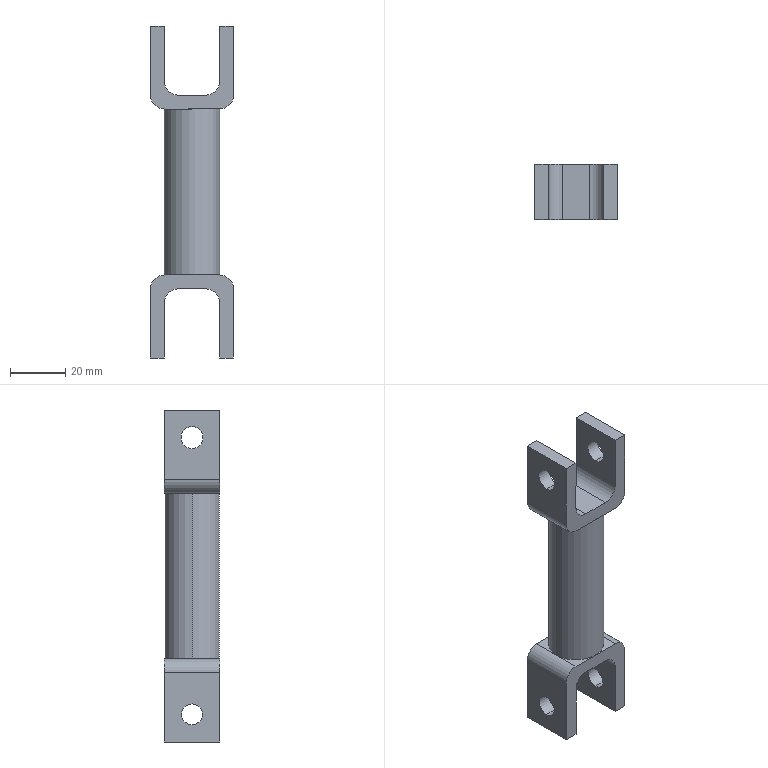Part | SolidWorks | features ICE 2, Extrusion 1 | 3 solids | 40 faces | box 30 x 20 x 120 mm | volume 33900 mm3 | plane 22 | cylinder 18 | commonest cylinder face diameters 10 x8 7.569 x4 7.979 x4 20 x2
STEP:
#1=CARTESIAN_POINT('',(10.,0.,60.));
#2=VERTEX_POINT('',#1);
#3=CARTESIAN_POINT('',(-10.,0.,60.));
#4=VERTEX_POINT('',#3);
#5=CARTESIAN_POINT('',(0.,0.,60.));
#6=DIRECTION('',(0.,0.,1.));
#7=DIRECTION('',(1.,0.,0.));
#8=AXIS2_PLACEMENT_3D('',#5,#6,#7);
#9=CIRCLE('',#8,10.);
#10=EDGE_CURVE('',#2,#4,#9,.T.);
#11=ORIENTED_EDGE('',*,*,#10,.F.);
#12=CARTESIAN_POINT('',(10.,0.,0.));
#13=VERTEX_POINT('',#12);
#14=CARTESIAN_POINT('',(10.,0.,60.));
#15=DIRECTION('',(0.,0.,-1.));
#16=VECTOR('',#15,1000.);
#17=LINE('',#14,#16);
#18=EDGE_CURVE('',#2,#13,#17,.T.);
#19=ORIENTED_EDGE('',*,*,#18,.T.);
#20=CARTESIAN_POINT('',(-10.,0.,0.));
#21=VERTEX_POINT('',#20);
#22=CARTESIAN_POINT('',(0.,0.,0.));
#23=DIRECTION('',(0.,0.,1.));
#24=DIRECTION('',(1.,0.,0.));
#25=AXIS2_PLACEMENT_3D('',#22,#23,#24);
#26=CIRCLE('',#25,10.);
#27=EDGE_CURVE('',#13,#21,#26,.T.);
#28=ORIENTED_EDGE('',*,*,#27,.T.);
#29=CARTESIAN_POINT('',(-10.,0.,60.));
#30=DIRECTION('',(0.,0.,-1.));
#31=VECTOR('',#30,1000.);
#32=LINE('',#29,#31);
#33=EDGE_CURVE('',#4,#21,#32,.T.);
#34=ORIENTED_EDGE('',*,*,#33,.F.);
#35=EDGE_LOOP('',(#11,#19,#28,#34));
#36=FACE_OUTER_BOUND('',#35,.T.);
#37=CARTESIAN_POINT('',(0.,0.,60.));
#38=DIRECTION('',(0.,0.,-1.));
#39=DIRECTION('',(-1.,0.,0.));
#40=AXIS2_PLACEMENT_3D('',#37,#38,#39);
#41=CYLINDRICAL_SURFACE('',#40,10.);
#42=ADVANCED_FACE('',(#36),#41,.T.);
#43=ORIENTED_EDGE('',*,*,#18,.F.);
#44=CARTESIAN_POINT('',(0.,0.,60.));
#45=DIRECTION('',(0.,0.,1.));
#46=DIRECTION('',(1.,0.,0.));
#47=AXIS2_PLACEMENT_3D('',#44,#45,#46);
#48=CIRCLE('',#47,10.);
#49=EDGE_CURVE('',#4,#2,#48,.T.);
#50=ORIENTED_EDGE('',*,*,#49,.F.);
#51=ORIENTED_EDGE('',*,*,#33,.T.);
#52=CARTESIAN_POINT('',(0.,0.,0.));
#53=DIRECTION('',(0.,0.,1.));
#54=DIRECTION('',(1.,0.,0.));
#55=AXIS2_PLACEMENT_3D('',#52,#53,#54);
#56=CIRCLE('',#55,10.);
#57=EDGE_CURVE('',#21,#13,#56,.T.);
#58=ORIENTED_EDGE('',*,*,#57,.T.);
#59=EDGE_LOOP('',(#43,#50,#51,#58));
#60=FACE_OUTER_BOUND('',#59,.T.);
#61=CARTESIAN_POINT('',(0.,0.,60.));
#62=DIRECTION('',(0.,0.,-1.));
#63=DIRECTION('',(-1.,0.,0.));
#64=AXIS2_PLACEMENT_3D('',#61,#62,#63);
#65=CYLINDRICAL_SURFACE('',#64,10.);
#66=ADVANCED_FACE('',(#60),#65,.T.);
#67=ORIENTED_EDGE('',*,*,#49,.T.);
#68=ORIENTED_EDGE('',*,*,#10,.T.);
#69=EDGE_LOOP('',(#67,#68));
#70=FACE_OUTER_BOUND('',#69,.T.);
#71=CARTESIAN_POINT('',(0.,0.,60.));
#72=DIRECTION('',(0.,0.,1.));
#73=DIRECTION('',(1.,0.,0.));
#74=AXIS2_PLACEMENT_3D('',#71,#72,#73);
#75=PLANE('',#74);
#76=ADVANCED_FACE('',(#70),#75,.T.);
#77=ORIENTED_EDGE('',*,*,#57,.F.);
#78=ORIENTED_EDGE('',*,*,#27,.F.);
#79=EDGE_LOOP('',(#77,#78));
#80=FACE_OUTER_BOUND('',#79,.T.);
#81=CARTESIAN_POINT('',(0.,0.,0.));
#82=DIRECTION('',(0.,0.,1.));
#83=DIRECTION('',(1.,0.,0.));
#84=AXIS2_PLACEMENT_3D('',#81,#82,#83);
#85=PLANE('',#84);
#86=ADVANCED_FACE('',(#80),#85,.F.);
#87=CLOSED_SHELL('',(#42,#66,#76,#86));
#88=MANIFOLD_SOLID_BREP('',#87);
#89=CARTESIAN_POINT('',(15.,0.,76.011));
#90=VERTEX_POINT('',#89);
#91=CARTESIAN_POINT('',(15.,0.,83.989));
#92=VERTEX_POINT('',#91);
#93=CARTESIAN_POINT('',(15.,0.,80.));
#94=DIRECTION('',(-1.,0.,0.));
#95=DIRECTION('',(0.,0.,1.));
#96=AXIS2_PLACEMENT_3D('',#93,#94,#95);
#97=CIRCLE('',#96,3.989);
#98=EDGE_CURVE('',#90,#92,#97,.T.);
#99=ORIENTED_EDGE('',*,*,#98,.F.);
#100=CARTESIAN_POINT('',(10.,0.,76.011));
#101=VERTEX_POINT('',#100);
#102=CARTESIAN_POINT('',(15.,0.,76.011));
#103=DIRECTION('',(-1.,0.,0.));
#104=VECTOR('',#103,1000.);
#105=LINE('',#102,#104);
#106=EDGE_CURVE('',#90,#101,#105,.T.);
#107=ORIENTED_EDGE('',*,*,#106,.T.);
#108=CARTESIAN_POINT('',(10.,0.,83.989));
#109=VERTEX_POINT('',#108);
#110=CARTESIAN_POINT('',(10.,0.,80.));
#111=DIRECTION('',(1.,0.,0.));
#112=DIRECTION('',(0.,0.,-1.));
#113=AXIS2_PLACEMENT_3D('',#110,#111,#112);
#114=CIRCLE('',#113,3.989);
#115=EDGE_CURVE('',#109,#101,#114,.T.);
#116=ORIENTED_EDGE('',*,*,#115,.F.);
#117=CARTESIAN_POINT('',(15.,0.,83.989));
#118=DIRECTION('',(-1.,0.,0.));
#119=VECTOR('',#118,1000.);
#120=LINE('',#117,#119);
#121=EDGE_CURVE('',#92,#109,#120,.T.);
#122=ORIENTED_EDGE('',*,*,#121,.F.);
#123=EDGE_LOOP('',(#99,#107,#116,#122));
#124=FACE_OUTER_BOUND('',#123,.T.);
#125=CARTESIAN_POINT('',(15.,0.,80.));
#126=DIRECTION('',(-1.,0.,0.));
#127=DIRECTION('',(0.,0.,1.));
#128=AXIS2_PLACEMENT_3D('',#125,#126,#127);
#129=CYLINDRICAL_SURFACE('',#128,3.989);
#130=ADVANCED_FACE('',(#124),#129,.F.);
#131=CARTESIAN_POINT('',(-10.,0.,76.011));
#132=VERTEX_POINT('',#131);
#133=CARTESIAN_POINT('',(-10.,0.,83.989));
#134=VERTEX_POINT('',#133);
#135=CARTESIAN_POINT('',(-10.,0.,80.));
#136=DIRECTION('',(-1.,0.,0.));
#137=DIRECTION('',(0.,0.,1.));
#138=AXIS2_PLACEMENT_3D('',#135,#136,#137);
#139=CIRCLE('',#138,3.989);
#140=EDGE_CURVE('',#132,#134,#139,.T.);
#141=ORIENTED_EDGE('',*,*,#140,.F.);
#142=CARTESIAN_POINT('',(-15.,0.,76.011));
#143=VERTEX_POINT('',#142);
#144=CARTESIAN_POINT('',(15.,0.,76.011));
#145=DIRECTION('',(-1.,0.,0.));
#146=VECTOR('',#145,1000.);
#147=LINE('',#144,#146);
#148=EDGE_CURVE('',#132,#143,#147,.T.);
#149=ORIENTED_EDGE('',*,*,#148,.T.);
#150=CARTESIAN_POINT('',(-15.,0.,83.989));
#151=VERTEX_POINT('',#150);
#152=CARTESIAN_POINT('',(-15.,0.,80.));
#153=DIRECTION('',(-1.,0.,0.));
#154=DIRECTION('',(0.,0.,1.));
#155=AXIS2_PLACEMENT_3D('',#152,#153,#154);
#156=CIRCLE('',#155,3.989);
#157=EDGE_CURVE('',#143,#151,#156,.T.);
#158=ORIENTED_EDGE('',*,*,#157,.T.);
#159=CARTESIAN_POINT('',(15.,0.,83.989));
#160=DIRECTION('',(-1.,0.,0.));
#161=VECTOR('',#160,1000.);
#162=LINE('',#159,#161);
#163=EDGE_CURVE('',#134,#151,#162,.T.);
#164=ORIENTED_EDGE('',*,*,#163,.F.);
#165=EDGE_LOOP('',(#141,#149,#158,#164));
#166=FACE_OUTER_BOUND('',#165,.T.);
#167=CARTESIAN_POINT('',(15.,0.,80.));
#168=DIRECTION('',(-1.,0.,0.));
#169=DIRECTION('',(0.,0.,1.));
#170=AXIS2_PLACEMENT_3D('',#167,#168,#169);
#171=CYLINDRICAL_SURFACE('',#170,3.989);
#172=ADVANCED_FACE('',(#166),#171,.F.);
#173=CARTESIAN_POINT('',(5.,-10.,65.));
#174=VERTEX_POINT('',#173);
#175=CARTESIAN_POINT('',(10.,-10.,70.));
#176=VERTEX_POINT('',#175);
#177=CARTESIAN_POINT('',(5.,-10.,70.));
#178=DIRECTION('',(0.,-1.,0.));
#179=DIRECTION('',(0.,0.,-1.));
#180=AXIS2_PLACEMENT_3D('',#177,#178,#179);
#181=CIRCLE('',#180,5.);
#182=EDGE_CURVE('',#174,#176,#181,.T.);
#183=ORIENTED_EDGE('',*,*,#182,.T.);
#184=CARTESIAN_POINT('',(10.,10.,70.));
#185=VERTEX_POINT('',#184);
#186=CARTESIAN_POINT('',(10.,10.,70.));
#187=DIRECTION('',(0.,-1.,0.));
#188=VECTOR('',#187,1000.);
#189=LINE('',#186,#188);
#190=EDGE_CURVE('',#185,#176,#189,.T.);
#191=ORIENTED_EDGE('',*,*,#190,.F.);
#192=CARTESIAN_POINT('',(5.,10.,65.));
#193=VERTEX_POINT('',#192);
#194=CARTESIAN_POINT('',(5.,10.,70.));
#195=DIRECTION('',(0.,-1.,0.));
#196=DIRECTION('',(0.,0.,-1.));
#197=AXIS2_PLACEMENT_3D('',#194,#195,#196);
#198=CIRCLE('',#197,5.);
#199=EDGE_CURVE('',#193,#185,#198,.T.);
#200=ORIENTED_EDGE('',*,*,#199,.F.);
#201=CARTESIAN_POINT('',(5.,10.,65.));
#202=DIRECTION('',(0.,-1.,0.));
#203=VECTOR('',#202,1000.);
#204=LINE('',#201,#203);
#205=EDGE_CURVE('',#193,#174,#204,.T.);
#206=ORIENTED_EDGE('',*,*,#205,.T.);
#207=EDGE_LOOP('',(#183,#191,#200,#206));
#208=FACE_OUTER_BOUND('',#207,.T.);
#209=CARTESIAN_POINT('',(5.,10.,70.));
#210=DIRECTION('',(0.,-1.,0.));
#211=DIRECTION('',(0.,0.,-1.));
#212=AXIS2_PLACEMENT_3D('',#209,#210,#211);
#213=CYLINDRICAL_SURFACE('',#212,5.);
#214=ADVANCED_FACE('',(#208),#213,.F.);
#215=ORIENTED_EDGE('',*,*,#115,.T.);
#216=CARTESIAN_POINT('',(10.,0.,80.));
#217=DIRECTION('',(1.,0.,0.));
#218=DIRECTION('',(0.,0.,-1.));
#219=AXIS2_PLACEMENT_3D('',#216,#217,#218);
#220=CIRCLE('',#219,3.989);
#221=EDGE_CURVE('',#101,#109,#220,.T.);
#222=ORIENTED_EDGE('',*,*,#221,.T.);
#223=EDGE_LOOP('',(#215,#222));
#224=FACE_BOUND('',#223,.T.);
#225=CARTESIAN_POINT('',(10.,-10.,90.));
#226=VERTEX_POINT('',#225);
#227=CARTESIAN_POINT('',(10.,-10.,70.));
#228=DIRECTION('',(0.,0.,1.));
#229=VECTOR('',#228,1000.);
#230=LINE('',#227,#229);
#231=EDGE_CURVE('',#176,#226,#230,.T.);
#232=ORIENTED_EDGE('',*,*,#231,.T.);
#233=CARTESIAN_POINT('',(10.,10.,90.));
#234=VERTEX_POINT('',#233);
#235=CARTESIAN_POINT('',(10.,10.,90.));
#236=DIRECTION('',(0.,-1.,0.));
#237=VECTOR('',#236,1000.);
#238=LINE('',#235,#237);
#239=EDGE_CURVE('',#234,#226,#238,.T.);
#240=ORIENTED_EDGE('',*,*,#239,.F.);
#241=CARTESIAN_POINT('',(10.,10.,70.));
#242=DIRECTION('',(0.,0.,1.));
#243=VECTOR('',#242,1000.);
#244=LINE('',#241,#243);
#245=EDGE_CURVE('',#185,#234,#244,.T.);
#246=ORIENTED_EDGE('',*,*,#245,.F.);
#247=ORIENTED_EDGE('',*,*,#190,.T.);
#248=EDGE_LOOP('',(#232,#240,#246,#247));
#249=FACE_OUTER_BOUND('',#248,.T.);
#250=CARTESIAN_POINT('',(10.,10.,70.));
#251=DIRECTION('',(1.,0.,0.));
#252=DIRECTION('',(0.,0.,-1.));
#253=AXIS2_PLACEMENT_3D('',#250,#251,#252);
#254=PLANE('',#253);
#255=ADVANCED_FACE('',(#224,#249),#254,.F.);
#256=CARTESIAN_POINT('',(15.,-10.,90.));
#257=VERTEX_POINT('',#256);
#258=CARTESIAN_POINT('',(10.,-10.,90.));
#259=DIRECTION('',(1.,0.,0.));
#260=VECTOR('',#259,1000.);
#261=LINE('',#258,#260);
#262=EDGE_CURVE('',#226,#257,#261,.T.);
#263=ORIENTED_EDGE('',*,*,#262,.T.);
#264=CARTESIAN_POINT('',(15.,10.,90.));
#265=VERTEX_POINT('',#264);
#266=CARTESIAN_POINT('',(15.,10.,90.));
#267=DIRECTION('',(0.,-1.,0.));
#268=VECTOR('',#267,1000.);
#269=LINE('',#266,#268);
#270=EDGE_CURVE('',#265,#257,#269,.T.);
#271=ORIENTED_EDGE('',*,*,#270,.F.);
#272=CARTESIAN_POINT('',(10.,10.,90.));
#273=DIRECTION('',(1.,0.,0.));
#274=VECTOR('',#273,1000.);
#275=LINE('',#272,#274);
#276=EDGE_CURVE('',#234,#265,#275,.T.);
#277=ORIENTED_EDGE('',*,*,#276,.F.);
#278=ORIENTED_EDGE('',*,*,#239,.T.);
#279=EDGE_LOOP('',(#263,#271,#277,#278));
#280=FACE_OUTER_BOUND('',#279,.T.);
#281=CARTESIAN_POINT('',(10.,10.,90.));
#282=DIRECTION('',(0.,0.,-1.));
#283=DIRECTION('',(-1.,0.,0.));
#284=AXIS2_PLACEMENT_3D('',#281,#282,#283);
#285=PLANE('',#284);
#286=ADVANCED_FACE('',(#280),#285,.F.);
#287=CARTESIAN_POINT('',(15.,0.,80.));
#288=DIRECTION('',(-1.,0.,0.));
#289=DIRECTION('',(0.,0.,1.));
#290=AXIS2_PLACEMENT_3D('',#287,#288,#289);
#291=CIRCLE('',#290,3.989);
#292=EDGE_CURVE('',#92,#90,#291,.T.);
#293=ORIENTED_EDGE('',*,*,#292,.T.);
#294=ORIENTED_EDGE('',*,*,#98,.T.);
#295=EDGE_LOOP('',(#293,#294));
#296=FACE_BOUND('',#295,.T.);
#297=CARTESIAN_POINT('',(15.,-10.,65.));
#298=VERTEX_POINT('',#297);
#299=CARTESIAN_POINT('',(15.,-10.,90.));
#300=DIRECTION('',(0.,0.,-1.));
#301=VECTOR('',#300,1000.);
#302=LINE('',#299,#301);
#303=EDGE_CURVE('',#257,#298,#302,.T.);
#304=ORIENTED_EDGE('',*,*,#303,.T.);
#305=CARTESIAN_POINT('',(15.,10.,65.));
#306=VERTEX_POINT('',#305);
#307=CARTESIAN_POINT('',(15.,10.,65.));
#308=DIRECTION('',(0.,-1.,0.));
#309=VECTOR('',#308,1000.);
#310=LINE('',#307,#309);
#311=EDGE_CURVE('',#306,#298,#310,.T.);
#312=ORIENTED_EDGE('',*,*,#311,.F.);
#313=CARTESIAN_POINT('',(15.,10.,90.));
#314=DIRECTION('',(0.,0.,-1.));
#315=VECTOR('',#314,1000.);
#316=LINE('',#313,#315);
#317=EDGE_CURVE('',#265,#306,#316,.T.);
#318=ORIENTED_EDGE('',*,*,#317,.F.);
#319=ORIENTED_EDGE('',*,*,#270,.T.);
#320=EDGE_LOOP('',(#304,#312,#318,#319));
#321=FACE_OUTER_BOUND('',#320,.T.);
#322=CARTESIAN_POINT('',(15.,10.,90.));
#323=DIRECTION('',(-1.,0.,0.));
#324=DIRECTION('',(0.,0.,1.));
#325=AXIS2_PLACEMENT_3D('',#322,#323,#324);
#326=PLANE('',#325);
#327=ADVANCED_FACE('',(#296,#321),#326,.F.);
#328=CARTESIAN_POINT('',(10.,-10.,60.));
#329=VERTEX_POINT('',#328);
#330=CARTESIAN_POINT('',(10.,-10.,65.));
#331=DIRECTION('',(0.,1.,0.));
#332=DIRECTION('',(0.,0.,-1.));
#333=AXIS2_PLACEMENT_3D('',#330,#331,#332);
#334=CIRCLE('',#333,5.);
#335=EDGE_CURVE('',#298,#329,#334,.T.);
#336=ORIENTED_EDGE('',*,*,#335,.T.);
#337=CARTESIAN_POINT('',(10.,10.,60.));
#338=VERTEX_POINT('',#337);
#339=CARTESIAN_POINT('',(10.,10.,60.));
#340=DIRECTION('',(0.,-1.,0.));
#341=VECTOR('',#340,1000.);
#342=LINE('',#339,#341);
#343=EDGE_CURVE('',#338,#329,#342,.T.);
#344=ORIENTED_EDGE('',*,*,#343,.F.);
#345=CARTESIAN_POINT('',(10.,10.,65.));
#346=DIRECTION('',(0.,1.,0.));
#347=DIRECTION('',(0.,0.,-1.));
#348=AXIS2_PLACEMENT_3D('',#345,#346,#347);
#349=CIRCLE('',#348,5.);
#350=EDGE_CURVE('',#306,#338,#349,.T.);
#351=ORIENTED_EDGE('',*,*,#350,.F.);
#352=ORIENTED_EDGE('',*,*,#311,.T.);
#353=EDGE_LOOP('',(#336,#344,#351,#352));
#354=FACE_OUTER_BOUND('',#353,.T.);
#355=CARTESIAN_POINT('',(10.,10.,65.));
#356=DIRECTION('',(0.,-1.,0.));
#357=DIRECTION('',(0.,0.,-1.));
#358=AXIS2_PLACEMENT_3D('',#355,#356,#357);
#359=CYLINDRICAL_SURFACE('',#358,5.);
#360=ADVANCED_FACE('',(#354),#359,.T.);
#361=CARTESIAN_POINT('',(-10.,-10.,60.));
#362=VERTEX_POINT('',#361);
#363=CARTESIAN_POINT('',(-10.,-10.,60.));
#364=DIRECTION('',(-1.,0.,0.));
#365=VECTOR('',#364,1000.);
#366=LINE('',#363,#365);
#367=EDGE_CURVE('',#329,#362,#366,.T.);
#368=ORIENTED_EDGE('',*,*,#367,.T.);
#369=CARTESIAN_POINT('',(-10.,10.,60.));
#370=VERTEX_POINT('',#369);
#371=CARTESIAN_POINT('',(-10.,10.,60.));
#372=DIRECTION('',(0.,-1.,0.));
#373=VECTOR('',#372,1000.);
#374=LINE('',#371,#373);
#375=EDGE_CURVE('',#370,#362,#374,.T.);
#376=ORIENTED_EDGE('',*,*,#375,.F.);
#377=CARTESIAN_POINT('',(-10.,10.,60.));
#378=DIRECTION('',(-1.,0.,0.));
#379=VECTOR('',#378,1000.);
#380=LINE('',#377,#379);
#381=EDGE_CURVE('',#338,#370,#380,.T.);
#382=ORIENTED_EDGE('',*,*,#381,.F.);
#383=ORIENTED_EDGE('',*,*,#343,.T.);
#384=EDGE_LOOP('',(#368,#376,#382,#383));
#385=FACE_OUTER_BOUND('',#384,.T.);
#386=CARTESIAN_POINT('',(-10.,10.,60.));
#387=DIRECTION('',(0.,0.,1.));
#388=DIRECTION('',(1.,0.,0.));
#389=AXIS2_PLACEMENT_3D('',#386,#387,#388);
#390=PLANE('',#389);
#391=ADVANCED_FACE('',(#385),#390,.F.);
#392=CARTESIAN_POINT('',(-15.,-10.,65.));
#393=VERTEX_POINT('',#392);
#394=CARTESIAN_POINT('',(-10.,-10.,65.));
#395=DIRECTION('',(0.,1.,0.));
#396=DIRECTION('',(0.,0.,-1.));
#397=AXIS2_PLACEMENT_3D('',#394,#395,#396);
#398=CIRCLE('',#397,5.);
#399=EDGE_CURVE('',#362,#393,#398,.T.);
#400=ORIENTED_EDGE('',*,*,#399,.T.);
#401=CARTESIAN_POINT('',(-15.,10.,65.));
#402=VERTEX_POINT('',#401);
#403=CARTESIAN_POINT('',(-15.,10.,65.));
#404=DIRECTION('',(0.,-1.,0.));
#405=VECTOR('',#404,1000.);
#406=LINE('',#403,#405);
#407=EDGE_CURVE('',#402,#393,#406,.T.);
#408=ORIENTED_EDGE('',*,*,#407,.F.);
#409=CARTESIAN_POINT('',(-10.,10.,65.));
#410=DIRECTION('',(0.,1.,0.));
#411=DIRECTION('',(0.,0.,-1.));
#412=AXIS2_PLACEMENT_3D('',#409,#410,#411);
#413=CIRCLE('',#412,5.);
#414=EDGE_CURVE('',#370,#402,#413,.T.);
#415=ORIENTED_EDGE('',*,*,#414,.F.);
#416=ORIENTED_EDGE('',*,*,#375,.T.);
#417=EDGE_LOOP('',(#400,#408,#415,#416));
#418=FACE_OUTER_BOUND('',#417,.T.);
#419=CARTESIAN_POINT('',(-10.,10.,65.));
#420=DIRECTION('',(0.,-1.,0.));
#421=DIRECTION('',(0.,0.,-1.));
#422=AXIS2_PLACEMENT_3D('',#419,#420,#421);
#423=CYLINDRICAL_SURFACE('',#422,5.);
#424=ADVANCED_FACE('',(#418),#423,.T.);
#425=CARTESIAN_POINT('',(-15.,0.,80.));
#426=DIRECTION('',(-1.,0.,0.));
#427=DIRECTION('',(0.,0.,1.));
#428=AXIS2_PLACEMENT_3D('',#425,#426,#427);
#429=CIRCLE('',#428,3.989);
#430=EDGE_CURVE('',#151,#143,#429,.T.);
#431=ORIENTED_EDGE('',*,*,#430,.F.);
#432=ORIENTED_EDGE('',*,*,#157,.F.);
#433=EDGE_LOOP('',(#431,#432));
#434=FACE_BOUND('',#433,.T.);
#435=CARTESIAN_POINT('',(-15.,-10.,90.));
#436=VERTEX_POINT('',#435);
#437=CARTESIAN_POINT('',(-15.,-10.,90.));
#438=DIRECTION('',(0.,0.,1.));
#439=VECTOR('',#438,1000.);
#440=LINE('',#437,#439);
#441=EDGE_CURVE('',#393,#436,#440,.T.);
#442=ORIENTED_EDGE('',*,*,#441,.T.);
#443=CARTESIAN_POINT('',(-15.,10.,90.));
#444=VERTEX_POINT('',#443);
#445=CARTESIAN_POINT('',(-15.,10.,90.));
#446=DIRECTION('',(0.,-1.,0.));
#447=VECTOR('',#446,1000.);
#448=LINE('',#445,#447);
#449=EDGE_CURVE('',#444,#436,#448,.T.);
#450=ORIENTED_EDGE('',*,*,#449,.F.);
#451=CARTESIAN_POINT('',(-15.,10.,90.));
#452=DIRECTION('',(0.,0.,1.));
#453=VECTOR('',#452,1000.);
#454=LINE('',#451,#453);
#455=EDGE_CURVE('',#402,#444,#454,.T.);
#456=ORIENTED_EDGE('',*,*,#455,.F.);
#457=ORIENTED_EDGE('',*,*,#407,.T.);
#458=EDGE_LOOP('',(#442,#450,#456,#457));
#459=FACE_OUTER_BOUND('',#458,.T.);
#460=CARTESIAN_POINT('',(-15.,10.,90.));
#461=DIRECTION('',(1.,0.,0.));
#462=DIRECTION('',(0.,0.,-1.));
#463=AXIS2_PLACEMENT_3D('',#460,#461,#462);
#464=PLANE('',#463);
#465=ADVANCED_FACE('',(#434,#459),#464,.F.);
#466=CARTESIAN_POINT('',(-10.,-10.,90.));
#467=VERTEX_POINT('',#466);
#468=CARTESIAN_POINT('',(-15.,-10.,90.));
#469=DIRECTION('',(1.,0.,0.));
#470=VECTOR('',#469,1000.);
#471=LINE('',#468,#470);
#472=EDGE_CURVE('',#436,#467,#471,.T.);
#473=ORIENTED_EDGE('',*,*,#472,.T.);
#474=CARTESIAN_POINT('',(-10.,10.,90.));
#475=VERTEX_POINT('',#474);
#476=CARTESIAN_POINT('',(-10.,10.,90.));
#477=DIRECTION('',(0.,-1.,0.));
#478=VECTOR('',#477,1000.);
#479=LINE('',#476,#478);
#480=EDGE_CURVE('',#475,#467,#479,.T.);
#481=ORIENTED_EDGE('',*,*,#480,.F.);
#482=CARTESIAN_POINT('',(-15.,10.,90.));
#483=DIRECTION('',(1.,0.,0.));
#484=VECTOR('',#483,1000.);
#485=LINE('',#482,#484);
#486=EDGE_CURVE('',#444,#475,#485,.T.);
#487=ORIENTED_EDGE('',*,*,#486,.F.);
#488=ORIENTED_EDGE('',*,*,#449,.T.);
#489=EDGE_LOOP('',(#473,#481,#487,#488));
#490=FACE_OUTER_BOUND('',#489,.T.);
#491=CARTESIAN_POINT('',(-15.,10.,90.));
#492=DIRECTION('',(0.,0.,-1.));
#493=DIRECTION('',(-1.,0.,0.));
#494=AXIS2_PLACEMENT_3D('',#491,#492,#493);
#495=PLANE('',#494);
#496=ADVANCED_FACE('',(#490),#495,.F.);
#497=CARTESIAN_POINT('',(-10.,0.,80.));
#498=DIRECTION('',(-1.,0.,0.));
#499=DIRECTION('',(0.,0.,1.));
#500=AXIS2_PLACEMENT_3D('',#497,#498,#499);
#501=CIRCLE('',#500,3.989);
#502=EDGE_CURVE('',#134,#132,#501,.T.);
#503=ORIENTED_EDGE('',*,*,#502,.T.);
#504=ORIENTED_EDGE('',*,*,#140,.T.);
#505=EDGE_LOOP('',(#503,#504));
#506=FACE_BOUND('',#505,.T.);
#507=CARTESIAN_POINT('',(-10.,-10.,70.));
#508=VERTEX_POINT('',#507);
#509=CARTESIAN_POINT('',(-10.,-10.,90.));
#510=DIRECTION('',(0.,0.,-1.));
#511=VECTOR('',#510,1000.);
#512=LINE('',#509,#511);
#513=EDGE_CURVE('',#467,#508,#512,.T.);
#514=ORIENTED_EDGE('',*,*,#513,.T.);
#515=CARTESIAN_POINT('',(-10.,10.,70.));
#516=VERTEX_POINT('',#515);
#517=CARTESIAN_POINT('',(-10.,10.,70.));
#518=DIRECTION('',(0.,-1.,0.));
#519=VECTOR('',#518,1000.);
#520=LINE('',#517,#519);
#521=EDGE_CURVE('',#516,#508,#520,.T.);
#522=ORIENTED_EDGE('',*,*,#521,.F.);
#523=CARTESIAN_POINT('',(-10.,10.,90.));
#524=DIRECTION('',(0.,0.,-1.));
#525=VECTOR('',#524,1000.);
#526=LINE('',#523,#525);
#527=EDGE_CURVE('',#475,#516,#526,.T.);
#528=ORIENTED_EDGE('',*,*,#527,.F.);
#529=ORIENTED_EDGE('',*,*,#480,.T.);
#530=EDGE_LOOP('',(#514,#522,#528,#529));
#531=FACE_OUTER_BOUND('',#530,.T.);
#532=CARTESIAN_POINT('',(-10.,10.,90.));
#533=DIRECTION('',(-1.,0.,0.));
#534=DIRECTION('',(0.,0.,1.));
#535=AXIS2_PLACEMENT_3D('',#532,#533,#534);
#536=PLANE('',#535);
#537=ADVANCED_FACE('',(#506,#531),#536,.F.);
#538=CARTESIAN_POINT('',(-5.,-10.,65.));
#539=VERTEX_POINT('',#538);
#540=CARTESIAN_POINT('',(-5.,-10.,70.));
#541=DIRECTION('',(0.,-1.,0.));
#542=DIRECTION('',(0.,0.,-1.));
#543=AXIS2_PLACEMENT_3D('',#540,#541,#542);
#544=CIRCLE('',#543,5.);
#545=EDGE_CURVE('',#508,#539,#544,.T.);
#546=ORIENTED_EDGE('',*,*,#545,.T.);
#547=CARTESIAN_POINT('',(-5.,10.,65.));
#548=VERTEX_POINT('',#547);
#549=CARTESIAN_POINT('',(-5.,10.,65.));
#550=DIRECTION('',(0.,-1.,0.));
#551=VECTOR('',#550,1000.);
#552=LINE('',#549,#551);
#553=EDGE_CURVE('',#548,#539,#552,.T.);
#554=ORIENTED_EDGE('',*,*,#553,.F.);
#555=CARTESIAN_POINT('',(-5.,10.,70.));
#556=DIRECTION('',(0.,-1.,0.));
#557=DIRECTION('',(0.,0.,-1.));
#558=AXIS2_PLACEMENT_3D('',#555,#556,#557);
#559=CIRCLE('',#558,5.);
#560=EDGE_CURVE('',#516,#548,#559,.T.);
#561=ORIENTED_EDGE('',*,*,#560,.F.);
#562=ORIENTED_EDGE('',*,*,#521,.T.);
#563=EDGE_LOOP('',(#546,#554,#561,#562));
#564=FACE_OUTER_BOUND('',#563,.T.);
#565=CARTESIAN_POINT('',(-5.,10.,70.));
#566=DIRECTION('',(0.,-1.,0.));
#567=DIRECTION('',(0.,0.,-1.));
#568=AXIS2_PLACEMENT_3D('',#565,#566,#567);
#569=CYLINDRICAL_SURFACE('',#568,5.);
#570=ADVANCED_FACE('',(#564),#569,.F.);
#571=CARTESIAN_POINT('',(-5.,-10.,65.));
#572=DIRECTION('',(1.,0.,0.));
#573=VECTOR('',#572,1000.);
#574=LINE('',#571,#573);
#575=EDGE_CURVE('',#539,#174,#574,.T.);
#576=ORIENTED_EDGE('',*,*,#575,.T.);
#577=ORIENTED_EDGE('',*,*,#205,.F.);
#578=CARTESIAN_POINT('',(-5.,10.,65.));
#579=DIRECTION('',(1.,0.,0.));
#580=VECTOR('',#579,1000.);
#581=LINE('',#578,#580);
#582=EDGE_CURVE('',#548,#193,#581,.T.);
#583=ORIENTED_EDGE('',*,*,#582,.F.);
#584=ORIENTED_EDGE('',*,*,#553,.T.);
#585=EDGE_LOOP('',(#576,#577,#583,#584));
#586=FACE_OUTER_BOUND('',#585,.T.);
#587=CARTESIAN_POINT('',(-5.,10.,65.));
#588=DIRECTION('',(0.,0.,-1.));
#589=DIRECTION('',(-1.,0.,0.));
#590=AXIS2_PLACEMENT_3D('',#587,#588,#589);
#591=PLANE('',#590);
#592=ADVANCED_FACE('',(#586),#591,.F.);
#593=ORIENTED_EDGE('',*,*,#199,.T.);
#594=ORIENTED_EDGE('',*,*,#245,.T.);
#595=ORIENTED_EDGE('',*,*,#276,.T.);
#596=ORIENTED_EDGE('',*,*,#317,.T.);
#597=ORIENTED_EDGE('',*,*,#350,.T.);
#598=ORIENTED_EDGE('',*,*,#381,.T.);
#599=ORIENTED_EDGE('',*,*,#414,.T.);
#600=ORIENTED_EDGE('',*,*,#455,.T.);
#601=ORIENTED_EDGE('',*,*,#486,.T.);
#602=ORIENTED_EDGE('',*,*,#527,.T.);
#603=ORIENTED_EDGE('',*,*,#560,.T.);
#604=ORIENTED_EDGE('',*,*,#582,.T.);
#605=EDGE_LOOP('',(#593,#594,#595,#596,#597,#598,#599,#600,#601,#602,#603,#604));
#606=FACE_OUTER_BOUND('',#605,.T.);
#607=CARTESIAN_POINT('',(5.,10.,70.));
#608=DIRECTION('',(0.,-1.,0.));
#609=DIRECTION('',(0.,0.,-1.));
#610=AXIS2_PLACEMENT_3D('',#607,#608,#609);
#611=PLANE('',#610);
#612=ADVANCED_FACE('',(#606),#611,.F.);
#613=ORIENTED_EDGE('',*,*,#182,.F.);
#614=ORIENTED_EDGE('',*,*,#575,.F.);
#615=ORIENTED_EDGE('',*,*,#545,.F.);
#616=ORIENTED_EDGE('',*,*,#513,.F.);
#617=ORIENTED_EDGE('',*,*,#472,.F.);
#618=ORIENTED_EDGE('',*,*,#441,.F.);
#619=ORIENTED_EDGE('',*,*,#399,.F.);
#620=ORIENTED_EDGE('',*,*,#367,.F.);
#621=ORIENTED_EDGE('',*,*,#335,.F.);
#622=ORIENTED_EDGE('',*,*,#303,.F.);
#623=ORIENTED_EDGE('',*,*,#262,.F.);
#624=ORIENTED_EDGE('',*,*,#231,.F.);
#625=EDGE_LOOP('',(#613,#614,#615,#616,#617,#618,#619,#620,#621,#622,#623,#624));
#626=FACE_OUTER_BOUND('',#625,.T.);
#627=CARTESIAN_POINT('',(5.,-10.,70.));
#628=DIRECTION('',(0.,-1.,0.));
#629=DIRECTION('',(0.,0.,-1.));
#630=AXIS2_PLACEMENT_3D('',#627,#628,#629);
#631=PLANE('',#630);
#632=ADVANCED_FACE('',(#626),#631,.T.);
#633=ORIENTED_EDGE('',*,*,#148,.F.);
#634=ORIENTED_EDGE('',*,*,#502,.F.);
#635=ORIENTED_EDGE('',*,*,#163,.T.);
#636=ORIENTED_EDGE('',*,*,#430,.T.);
#637=EDGE_LOOP('',(#633,#634,#635,#636));
#638=FACE_OUTER_BOUND('',#637,.T.);
#639=CARTESIAN_POINT('',(15.,0.,80.));
#640=DIRECTION('',(-1.,0.,0.));
#641=DIRECTION('',(0.,0.,1.));
#642=AXIS2_PLACEMENT_3D('',#639,#640,#641);
#643=CYLINDRICAL_SURFACE('',#642,3.989);
#644=ADVANCED_FACE('',(#638),#643,.F.);
#645=ORIENTED_EDGE('',*,*,#106,.F.);
#646=ORIENTED_EDGE('',*,*,#292,.F.);
#647=ORIENTED_EDGE('',*,*,#121,.T.);
#648=ORIENTED_EDGE('',*,*,#221,.F.);
#649=EDGE_LOOP('',(#645,#646,#647,#648));
#650=FACE_OUTER_BOUND('',#649,.T.);
#651=CARTESIAN_POINT('',(15.,0.,80.));
#652=DIRECTION('',(-1.,0.,0.));
#653=DIRECTION('',(0.,0.,1.));
#654=AXIS2_PLACEMENT_3D('',#651,#652,#653);
#655=CYLINDRICAL_SURFACE('',#654,3.989);
#656=ADVANCED_FACE('',(#650),#655,.F.);
#657=CLOSED_SHELL('',(#130,#172,#214,#255,#286,#327,#360,#391,#424,#465,#496,#537,#570,#592,#612,#632,#644,#656));
#658=MANIFOLD_SOLID_BREP('',#657);
#659=CARTESIAN_POINT('',(15.,0.,-23.784));
#660=VERTEX_POINT('',#659);
#661=CARTESIAN_POINT('',(15.,0.,-16.216));
#662=VERTEX_POINT('',#661);
#663=CARTESIAN_POINT('',(15.,0.,-20.));
#664=DIRECTION('',(-1.,0.,0.));
#665=DIRECTION('',(0.,0.,1.));
#666=AXIS2_PLACEMENT_3D('',#663,#664,#665);
#667=CIRCLE('',#666,3.784);
#668=EDGE_CURVE('',#660,#662,#667,.T.);
#669=ORIENTED_EDGE('',*,*,#668,.F.);
#670=CARTESIAN_POINT('',(10.,0.,-23.784));
#671=VERTEX_POINT('',#670);
#672=CARTESIAN_POINT('',(15.,0.,-23.784));
#673=DIRECTION('',(-1.,0.,0.));
#674=VECTOR('',#673,1000.);
#675=LINE('',#672,#674);
#676=EDGE_CURVE('',#660,#671,#675,.T.);
#677=ORIENTED_EDGE('',*,*,#676,.T.);
#678=CARTESIAN_POINT('',(10.,0.,-16.216));
#679=VERTEX_POINT('',#678);
#680=CARTESIAN_POINT('',(10.,0.,-20.));
#681=DIRECTION('',(1.,0.,0.));
#682=DIRECTION('',(0.,0.,-1.));
#683=AXIS2_PLACEMENT_3D('',#680,#681,#682);
#684=CIRCLE('',#683,3.784);
#685=EDGE_CURVE('',#679,#671,#684,.T.);
#686=ORIENTED_EDGE('',*,*,#685,.F.);
#687=CARTESIAN_POINT('',(15.,0.,-16.216));
#688=DIRECTION('',(-1.,0.,0.));
#689=VECTOR('',#688,1000.);
#690=LINE('',#687,#689);
#691=EDGE_CURVE('',#662,#679,#690,.T.);
#692=ORIENTED_EDGE('',*,*,#691,.F.);
#693=EDGE_LOOP('',(#669,#677,#686,#692));
#694=FACE_OUTER_BOUND('',#693,.T.);
#695=CARTESIAN_POINT('',(15.,0.,-20.));
#696=DIRECTION('',(-1.,0.,0.));
#697=DIRECTION('',(0.,0.,1.));
#698=AXIS2_PLACEMENT_3D('',#695,#696,#697);
#699=CYLINDRICAL_SURFACE('',#698,3.784);
#700=ADVANCED_FACE('',(#694),#699,.F.);
#701=CARTESIAN_POINT('',(-10.,0.,-23.784));
#702=VERTEX_POINT('',#701);
#703=CARTESIAN_POINT('',(-10.,0.,-16.216));
#704=VERTEX_POINT('',#703);
#705=CARTESIAN_POINT('',(-10.,0.,-20.));
#706=DIRECTION('',(-1.,0.,0.));
#707=DIRECTION('',(0.,0.,1.));
#708=AXIS2_PLACEMENT_3D('',#705,#706,#707);
#709=CIRCLE('',#708,3.784);
#710=EDGE_CURVE('',#702,#704,#709,.T.);
#711=ORIENTED_EDGE('',*,*,#710,.F.);
#712=CARTESIAN_POINT('',(-15.,0.,-23.784));
#713=VERTEX_POINT('',#712);
#714=CARTESIAN_POINT('',(15.,0.,-23.784));
#715=DIRECTION('',(-1.,0.,0.));
#716=VECTOR('',#715,1000.);
#717=LINE('',#714,#716);
#718=EDGE_CURVE('',#702,#713,#717,.T.);
#719=ORIENTED_EDGE('',*,*,#718,.T.);
#720=CARTESIAN_POINT('',(-15.,0.,-16.216));
#721=VERTEX_POINT('',#720);
#722=CARTESIAN_POINT('',(-15.,0.,-20.));
#723=DIRECTION('',(-1.,0.,0.));
#724=DIRECTION('',(0.,0.,1.));
#725=AXIS2_PLACEMENT_3D('',#722,#723,#724);
#726=CIRCLE('',#725,3.784);
#727=EDGE_CURVE('',#713,#721,#726,.T.);
#728=ORIENTED_EDGE('',*,*,#727,.T.);
#729=CARTESIAN_POINT('',(15.,0.,-16.216));
#730=DIRECTION('',(-1.,0.,0.));
#731=VECTOR('',#730,1000.);
#732=LINE('',#729,#731);
#733=EDGE_CURVE('',#704,#721,#732,.T.);
#734=ORIENTED_EDGE('',*,*,#733,.F.);
#735=EDGE_LOOP('',(#711,#719,#728,#734));
#736=FACE_OUTER_BOUND('',#735,.T.);
#737=CARTESIAN_POINT('',(15.,0.,-20.));
#738=DIRECTION('',(-1.,0.,0.));
#739=DIRECTION('',(0.,0.,1.));
#740=AXIS2_PLACEMENT_3D('',#737,#738,#739);
#741=CYLINDRICAL_SURFACE('',#740,3.784);
#742=ADVANCED_FACE('',(#736),#741,.F.);
#743=CARTESIAN_POINT('',(-15.,0.,-20.));
#744=DIRECTION('',(-1.,0.,0.));
#745=DIRECTION('',(0.,0.,1.));
#746=AXIS2_PLACEMENT_3D('',#743,#744,#745);
#747=CIRCLE('',#746,3.784);
#748=EDGE_CURVE('',#721,#713,#747,.T.);
#749=ORIENTED_EDGE('',*,*,#748,.F.);
#750=ORIENTED_EDGE('',*,*,#727,.F.);
#751=EDGE_LOOP('',(#749,#750));
#752=FACE_BOUND('',#751,.T.);
#753=CARTESIAN_POINT('',(-15.,-10.,-30.));
#754=VERTEX_POINT('',#753);
#755=CARTESIAN_POINT('',(-15.,-10.,-5.));
#756=VERTEX_POINT('',#755);
#757=CARTESIAN_POINT('',(-15.,-10.,-30.));
#758=DIRECTION('',(0.,0.,1.));
#759=VECTOR('',#758,1000.);
#760=LINE('',#757,#759);
#761=EDGE_CURVE('',#754,#756,#760,.T.);
#762=ORIENTED_EDGE('',*,*,#761,.T.);
#763=CARTESIAN_POINT('',(-15.,10.,-5.));
#764=VERTEX_POINT('',#763);
#765=CARTESIAN_POINT('',(-15.,10.,-5.));
#766=DIRECTION('',(0.,-1.,0.));
#767=VECTOR('',#766,1000.);
#768=LINE('',#765,#767);
#769=EDGE_CURVE('',#764,#756,#768,.T.);
#770=ORIENTED_EDGE('',*,*,#769,.F.);
#771=CARTESIAN_POINT('',(-15.,10.,-30.));
#772=VERTEX_POINT('',#771);
#773=CARTESIAN_POINT('',(-15.,10.,-30.));
#774=DIRECTION('',(0.,0.,1.));
#775=VECTOR('',#774,1000.);
#776=LINE('',#773,#775);
#777=EDGE_CURVE('',#772,#764,#776,.T.);
#778=ORIENTED_EDGE('',*,*,#777,.F.);
#779=CARTESIAN_POINT('',(-15.,10.,-30.));
#780=DIRECTION('',(0.,-1.,0.));
#781=VECTOR('',#780,1000.);
#782=LINE('',#779,#781);
#783=EDGE_CURVE('',#772,#754,#782,.T.);
#784=ORIENTED_EDGE('',*,*,#783,.T.);
#785=EDGE_LOOP('',(#762,#770,#778,#784));
#786=FACE_OUTER_BOUND('',#785,.T.);
#787=CARTESIAN_POINT('',(-15.,10.,-30.));
#788=DIRECTION('',(1.,0.,0.));
#789=DIRECTION('',(0.,0.,-1.));
#790=AXIS2_PLACEMENT_3D('',#787,#788,#789);
#791=PLANE('',#790);
#792=ADVANCED_FACE('',(#752,#786),#791,.F.);
#793=CARTESIAN_POINT('',(-10.,-10.,0.));
#794=VERTEX_POINT('',#793);
#795=CARTESIAN_POINT('',(-10.,-10.,-5.));
#796=DIRECTION('',(0.,1.,0.));
#797=DIRECTION('',(0.,0.,1.));
#798=AXIS2_PLACEMENT_3D('',#795,#796,#797);
#799=CIRCLE('',#798,5.);
#800=EDGE_CURVE('',#756,#794,#799,.T.);
#801=ORIENTED_EDGE('',*,*,#800,.T.);
#802=CARTESIAN_POINT('',(-10.,10.,0.));
#803=VERTEX_POINT('',#802);
#804=CARTESIAN_POINT('',(-10.,10.,0.));
#805=DIRECTION('',(0.,-1.,0.));
#806=VECTOR('',#805,1000.);
#807=LINE('',#804,#806);
#808=EDGE_CURVE('',#803,#794,#807,.T.);
#809=ORIENTED_EDGE('',*,*,#808,.F.);
#810=CARTESIAN_POINT('',(-10.,10.,-5.));
#811=DIRECTION('',(0.,1.,0.));
#812=DIRECTION('',(0.,0.,1.));
#813=AXIS2_PLACEMENT_3D('',#810,#811,#812);
#814=CIRCLE('',#813,5.);
#815=EDGE_CURVE('',#764,#803,#814,.T.);
#816=ORIENTED_EDGE('',*,*,#815,.F.);
#817=ORIENTED_EDGE('',*,*,#769,.T.);
#818=EDGE_LOOP('',(#801,#809,#816,#817));
#819=FACE_OUTER_BOUND('',#818,.T.);
#820=CARTESIAN_POINT('',(-10.,10.,-5.));
#821=DIRECTION('',(0.,-1.,0.));
#822=DIRECTION('',(0.,0.,-1.));
#823=AXIS2_PLACEMENT_3D('',#820,#821,#822);
#824=CYLINDRICAL_SURFACE('',#823,5.);
#825=ADVANCED_FACE('',(#819),#824,.T.);
#826=CARTESIAN_POINT('',(10.,-10.,0.));
#827=VERTEX_POINT('',#826);
#828=CARTESIAN_POINT('',(-10.,-10.,0.));
#829=DIRECTION('',(1.,0.,0.));
#830=VECTOR('',#829,1000.);
#831=LINE('',#828,#830);
#832=EDGE_CURVE('',#794,#827,#831,.T.);
#833=ORIENTED_EDGE('',*,*,#832,.T.);
#834=CARTESIAN_POINT('',(10.,10.,0.));
#835=VERTEX_POINT('',#834);
#836=CARTESIAN_POINT('',(10.,10.,0.));
#837=DIRECTION('',(0.,-1.,0.));
#838=VECTOR('',#837,1000.);
#839=LINE('',#836,#838);
#840=EDGE_CURVE('',#835,#827,#839,.T.);
#841=ORIENTED_EDGE('',*,*,#840,.F.);
#842=CARTESIAN_POINT('',(-10.,10.,0.));
#843=DIRECTION('',(1.,0.,0.));
#844=VECTOR('',#843,1000.);
#845=LINE('',#842,#844);
#846=EDGE_CURVE('',#803,#835,#845,.T.);
#847=ORIENTED_EDGE('',*,*,#846,.F.);
#848=ORIENTED_EDGE('',*,*,#808,.T.);
#849=EDGE_LOOP('',(#833,#841,#847,#848));
#850=FACE_OUTER_BOUND('',#849,.T.);
#851=CARTESIAN_POINT('',(-10.,10.,0.));
#852=DIRECTION('',(0.,0.,-1.));
#853=DIRECTION('',(-1.,0.,0.));
#854=AXIS2_PLACEMENT_3D('',#851,#852,#853);
#855=PLANE('',#854);
#856=ADVANCED_FACE('',(#850),#855,.F.);
#857=CARTESIAN_POINT('',(15.,-10.,-5.));
#858=VERTEX_POINT('',#857);
#859=CARTESIAN_POINT('',(10.,-10.,-5.));
#860=DIRECTION('',(0.,1.,0.));
#861=DIRECTION('',(0.,0.,1.));
#862=AXIS2_PLACEMENT_3D('',#859,#860,#861);
#863=CIRCLE('',#862,5.);
#864=EDGE_CURVE('',#827,#858,#863,.T.);
#865=ORIENTED_EDGE('',*,*,#864,.T.);
#866=CARTESIAN_POINT('',(15.,10.,-5.));
#867=VERTEX_POINT('',#866);
#868=CARTESIAN_POINT('',(15.,10.,-5.));
#869=DIRECTION('',(0.,-1.,0.));
#870=VECTOR('',#869,1000.);
#871=LINE('',#868,#870);
#872=EDGE_CURVE('',#867,#858,#871,.T.);
#873=ORIENTED_EDGE('',*,*,#872,.F.);
#874=CARTESIAN_POINT('',(10.,10.,-5.));
#875=DIRECTION('',(0.,1.,0.));
#876=DIRECTION('',(0.,0.,1.));
#877=AXIS2_PLACEMENT_3D('',#874,#875,#876);
#878=CIRCLE('',#877,5.);
#879=EDGE_CURVE('',#835,#867,#878,.T.);
#880=ORIENTED_EDGE('',*,*,#879,.F.);
#881=ORIENTED_EDGE('',*,*,#840,.T.);
#882=EDGE_LOOP('',(#865,#873,#880,#881));
#883=FACE_OUTER_BOUND('',#882,.T.);
#884=CARTESIAN_POINT('',(10.,10.,-5.));
#885=DIRECTION('',(0.,-1.,0.));
#886=DIRECTION('',(0.,0.,-1.));
#887=AXIS2_PLACEMENT_3D('',#884,#885,#886);
#888=CYLINDRICAL_SURFACE('',#887,5.);
#889=ADVANCED_FACE('',(#883),#888,.T.);
#890=CARTESIAN_POINT('',(15.,0.,-20.));
#891=DIRECTION('',(-1.,0.,0.));
#892=DIRECTION('',(0.,0.,1.));
#893=AXIS2_PLACEMENT_3D('',#890,#891,#892);
#894=CIRCLE('',#893,3.784);
#895=EDGE_CURVE('',#662,#660,#894,.T.);
#896=ORIENTED_EDGE('',*,*,#895,.T.);
#897=ORIENTED_EDGE('',*,*,#668,.T.);
#898=EDGE_LOOP('',(#896,#897));
#899=FACE_BOUND('',#898,.T.);
#900=CARTESIAN_POINT('',(15.,-10.,-30.));
#901=VERTEX_POINT('',#900);
#902=CARTESIAN_POINT('',(15.,-10.,-30.));
#903=DIRECTION('',(0.,0.,-1.));
#904=VECTOR('',#903,1000.);
#905=LINE('',#902,#904);
#906=EDGE_CURVE('',#858,#901,#905,.T.);
#907=ORIENTED_EDGE('',*,*,#906,.T.);
#908=CARTESIAN_POINT('',(15.,10.,-30.));
#909=VERTEX_POINT('',#908);
#910=CARTESIAN_POINT('',(15.,10.,-30.));
#911=DIRECTION('',(0.,-1.,0.));
#912=VECTOR('',#911,1000.);
#913=LINE('',#910,#912);
#914=EDGE_CURVE('',#909,#901,#913,.T.);
#915=ORIENTED_EDGE('',*,*,#914,.F.);
#916=CARTESIAN_POINT('',(15.,10.,-30.));
#917=DIRECTION('',(0.,0.,-1.));
#918=VECTOR('',#917,1000.);
#919=LINE('',#916,#918);
#920=EDGE_CURVE('',#867,#909,#919,.T.);
#921=ORIENTED_EDGE('',*,*,#920,.F.);
#922=ORIENTED_EDGE('',*,*,#872,.T.);
#923=EDGE_LOOP('',(#907,#915,#921,#922));
#924=FACE_OUTER_BOUND('',#923,.T.);
#925=CARTESIAN_POINT('',(15.,10.,-30.));
#926=DIRECTION('',(-1.,0.,0.));
#927=DIRECTION('',(0.,0.,1.));
#928=AXIS2_PLACEMENT_3D('',#925,#926,#927);
#929=PLANE('',#928);
#930=ADVANCED_FACE('',(#899,#924),#929,.F.);
#931=CARTESIAN_POINT('',(10.,-10.,-30.));
#932=VERTEX_POINT('',#931);
#933=CARTESIAN_POINT('',(10.,-10.,-30.));
#934=DIRECTION('',(-1.,0.,0.));
#935=VECTOR('',#934,1000.);
#936=LINE('',#933,#935);
#937=EDGE_CURVE('',#901,#932,#936,.T.);
#938=ORIENTED_EDGE('',*,*,#937,.T.);
#939=CARTESIAN_POINT('',(10.,10.,-30.));
#940=VERTEX_POINT('',#939);
#941=CARTESIAN_POINT('',(10.,10.,-30.));
#942=DIRECTION('',(0.,-1.,0.));
#943=VECTOR('',#942,1000.);
#944=LINE('',#941,#943);
#945=EDGE_CURVE('',#940,#932,#944,.T.);
#946=ORIENTED_EDGE('',*,*,#945,.F.);
#947=CARTESIAN_POINT('',(10.,10.,-30.));
#948=DIRECTION('',(-1.,0.,0.));
#949=VECTOR('',#948,1000.);
#950=LINE('',#947,#949);
#951=EDGE_CURVE('',#909,#940,#950,.T.);
#952=ORIENTED_EDGE('',*,*,#951,.F.);
#953=ORIENTED_EDGE('',*,*,#914,.T.);
#954=EDGE_LOOP('',(#938,#946,#952,#953));
#955=FACE_OUTER_BOUND('',#954,.T.);
#956=CARTESIAN_POINT('',(10.,10.,-30.));
#957=DIRECTION('',(0.,0.,1.));
#958=DIRECTION('',(1.,0.,0.));
#959=AXIS2_PLACEMENT_3D('',#956,#957,#958);
#960=PLANE('',#959);
#961=ADVANCED_FACE('',(#955),#960,.F.);
#962=ORIENTED_EDGE('',*,*,#685,.T.);
#963=CARTESIAN_POINT('',(10.,0.,-20.));
#964=DIRECTION('',(1.,0.,0.));
#965=DIRECTION('',(0.,0.,-1.));
#966=AXIS2_PLACEMENT_3D('',#963,#964,#965);
#967=CIRCLE('',#966,3.784);
#968=EDGE_CURVE('',#671,#679,#967,.T.);
#969=ORIENTED_EDGE('',*,*,#968,.T.);
#970=EDGE_LOOP('',(#962,#969));
#971=FACE_BOUND('',#970,.T.);
#972=CARTESIAN_POINT('',(10.,-10.,-10.));
#973=VERTEX_POINT('',#972);
#974=CARTESIAN_POINT('',(10.,-10.,-10.));
#975=DIRECTION('',(0.,0.,1.));
#976=VECTOR('',#975,1000.);
#977=LINE('',#974,#976);
#978=EDGE_CURVE('',#932,#973,#977,.T.);
#979=ORIENTED_EDGE('',*,*,#978,.T.);
#980=CARTESIAN_POINT('',(10.,10.,-10.));
#981=VERTEX_POINT('',#980);
#982=CARTESIAN_POINT('',(10.,10.,-10.));
#983=DIRECTION('',(0.,-1.,0.));
#984=VECTOR('',#983,1000.);
#985=LINE('',#982,#984);
#986=EDGE_CURVE('',#981,#973,#985,.T.);
#987=ORIENTED_EDGE('',*,*,#986,.F.);
#988=CARTESIAN_POINT('',(10.,10.,-10.));
#989=DIRECTION('',(0.,0.,1.));
#990=VECTOR('',#989,1000.);
#991=LINE('',#988,#990);
#992=EDGE_CURVE('',#940,#981,#991,.T.);
#993=ORIENTED_EDGE('',*,*,#992,.F.);
#994=ORIENTED_EDGE('',*,*,#945,.T.);
#995=EDGE_LOOP('',(#979,#987,#993,#994));
#996=FACE_OUTER_BOUND('',#995,.T.);
#997=CARTESIAN_POINT('',(10.,10.,-10.));
#998=DIRECTION('',(1.,0.,0.));
#999=DIRECTION('',(0.,0.,-1.));
#1000=AXIS2_PLACEMENT_3D('',#997,#998,#999);
#1001=PLANE('',#1000);
#1002=ADVANCED_FACE('',(#971,#996),#1001,.F.);
#1003=CARTESIAN_POINT('',(5.,-10.,-5.));
#1004=VERTEX_POINT('',#1003);
#1005=CARTESIAN_POINT('',(5.,-10.,-10.));
#1006=DIRECTION('',(0.,-1.,0.));
#1007=DIRECTION('',(0.,0.,1.));
#1008=AXIS2_PLACEMENT_3D('',#1005,#1006,#1007);
#1009=CIRCLE('',#1008,5.);
#1010=EDGE_CURVE('',#973,#1004,#1009,.T.);
#1011=ORIENTED_EDGE('',*,*,#1010,.T.);
#1012=CARTESIAN_POINT('',(5.,10.,-5.));
#1013=VERTEX_POINT('',#1012);
#1014=CARTESIAN_POINT('',(5.,10.,-5.));
#1015=DIRECTION('',(0.,-1.,0.));
#1016=VECTOR('',#1015,1000.);
#1017=LINE('',#1014,#1016);
#1018=EDGE_CURVE('',#1013,#1004,#1017,.T.);
#1019=ORIENTED_EDGE('',*,*,#1018,.F.);
#1020=CARTESIAN_POINT('',(5.,10.,-10.));
#1021=DIRECTION('',(0.,-1.,0.));
#1022=DIRECTION('',(0.,0.,1.));
#1023=AXIS2_PLACEMENT_3D('',#1020,#1021,#1022);
#1024=CIRCLE('',#1023,5.);
#1025=EDGE_CURVE('',#981,#1013,#1024,.T.);
#1026=ORIENTED_EDGE('',*,*,#1025,.F.);
#1027=ORIENTED_EDGE('',*,*,#986,.T.);
#1028=EDGE_LOOP('',(#1011,#1019,#1026,#1027));
#1029=FACE_OUTER_BOUND('',#1028,.T.);
#1030=CARTESIAN_POINT('',(5.,10.,-10.));
#1031=DIRECTION('',(0.,-1.,0.));
#1032=DIRECTION('',(0.,0.,-1.));
#1033=AXIS2_PLACEMENT_3D('',#1030,#1031,#1032);
#1034=CYLINDRICAL_SURFACE('',#1033,5.);
#1035=ADVANCED_FACE('',(#1029),#1034,.F.);
#1036=CARTESIAN_POINT('',(-5.,-10.,-5.));
#1037=VERTEX_POINT('',#1036);
#1038=CARTESIAN_POINT('',(-5.,-10.,-5.));
#1039=DIRECTION('',(-1.,0.,0.));
#1040=VECTOR('',#1039,1000.);
#1041=LINE('',#1038,#1040);
#1042=EDGE_CURVE('',#1004,#1037,#1041,.T.);
#1043=ORIENTED_EDGE('',*,*,#1042,.T.);
#1044=CARTESIAN_POINT('',(-5.,10.,-5.));
#1045=VERTEX_POINT('',#1044);
#1046=CARTESIAN_POINT('',(-5.,10.,-5.));
#1047=DIRECTION('',(0.,-1.,0.));
#1048=VECTOR('',#1047,1000.);
#1049=LINE('',#1046,#1048);
#1050=EDGE_CURVE('',#1045,#1037,#1049,.T.);
#1051=ORIENTED_EDGE('',*,*,#1050,.F.);
#1052=CARTESIAN_POINT('',(-5.,10.,-5.));
#1053=DIRECTION('',(-1.,0.,0.));
#1054=VECTOR('',#1053,1000.);
#1055=LINE('',#1052,#1054);
#1056=EDGE_CURVE('',#1013,#1045,#1055,.T.);
#1057=ORIENTED_EDGE('',*,*,#1056,.F.);
#1058=ORIENTED_EDGE('',*,*,#1018,.T.);
#1059=EDGE_LOOP('',(#1043,#1051,#1057,#1058));
#1060=FACE_OUTER_BOUND('',#1059,.T.);
#1061=CARTESIAN_POINT('',(-5.,10.,-5.));
#1062=DIRECTION('',(0.,0.,1.));
#1063=DIRECTION('',(1.,0.,0.));
#1064=AXIS2_PLACEMENT_3D('',#1061,#1062,#1063);
#1065=PLANE('',#1064);
#1066=ADVANCED_FACE('',(#1060),#1065,.F.);
#1067=CARTESIAN_POINT('',(-10.,-10.,-10.));
#1068=VERTEX_POINT('',#1067);
#1069=CARTESIAN_POINT('',(-5.,-10.,-10.));
#1070=DIRECTION('',(0.,-1.,0.));
#1071=DIRECTION('',(0.,0.,1.));
#1072=AXIS2_PLACEMENT_3D('',#1069,#1070,#1071);
#1073=CIRCLE('',#1072,5.);
#1074=EDGE_CURVE('',#1037,#1068,#1073,.T.);
#1075=ORIENTED_EDGE('',*,*,#1074,.T.);
#1076=CARTESIAN_POINT('',(-10.,10.,-10.));
#1077=VERTEX_POINT('',#1076);
#1078=CARTESIAN_POINT('',(-10.,10.,-10.));
#1079=DIRECTION('',(0.,-1.,0.));
#1080=VECTOR('',#1079,1000.);
#1081=LINE('',#1078,#1080);
#1082=EDGE_CURVE('',#1077,#1068,#1081,.T.);
#1083=ORIENTED_EDGE('',*,*,#1082,.F.);
#1084=CARTESIAN_POINT('',(-5.,10.,-10.));
#1085=DIRECTION('',(0.,-1.,0.));
#1086=DIRECTION('',(0.,0.,1.));
#1087=AXIS2_PLACEMENT_3D('',#1084,#1085,#1086);
#1088=CIRCLE('',#1087,5.);
#1089=EDGE_CURVE('',#1045,#1077,#1088,.T.);
#1090=ORIENTED_EDGE('',*,*,#1089,.F.);
#1091=ORIENTED_EDGE('',*,*,#1050,.T.);
#1092=EDGE_LOOP('',(#1075,#1083,#1090,#1091));
#1093=FACE_OUTER_BOUND('',#1092,.T.);
#1094=CARTESIAN_POINT('',(-5.,10.,-10.));
#1095=DIRECTION('',(0.,-1.,0.));
#1096=DIRECTION('',(0.,0.,-1.));
#1097=AXIS2_PLACEMENT_3D('',#1094,#1095,#1096);
#1098=CYLINDRICAL_SURFACE('',#1097,5.);
#1099=ADVANCED_FACE('',(#1093),#1098,.F.);
#1100=CARTESIAN_POINT('',(-10.,0.,-20.));
#1101=DIRECTION('',(-1.,0.,0.));
#1102=DIRECTION('',(0.,0.,1.));
#1103=AXIS2_PLACEMENT_3D('',#1100,#1101,#1102);
#1104=CIRCLE('',#1103,3.784);
#1105=EDGE_CURVE('',#704,#702,#1104,.T.);
#1106=ORIENTED_EDGE('',*,*,#1105,.T.);
#1107=ORIENTED_EDGE('',*,*,#710,.T.);
#1108=EDGE_LOOP('',(#1106,#1107));
#1109=FACE_BOUND('',#1108,.T.);
#1110=CARTESIAN_POINT('',(-10.,-10.,-30.));
#1111=VERTEX_POINT('',#1110);
#1112=CARTESIAN_POINT('',(-10.,-10.,-30.));
#1113=DIRECTION('',(0.,0.,-1.));
#1114=VECTOR('',#1113,1000.);
#1115=LINE('',#1112,#1114);
#1116=EDGE_CURVE('',#1068,#1111,#1115,.T.);
#1117=ORIENTED_EDGE('',*,*,#1116,.T.);
#1118=CARTESIAN_POINT('',(-10.,10.,-30.));
#1119=VERTEX_POINT('',#1118);
#1120=CARTESIAN_POINT('',(-10.,10.,-30.));
#1121=DIRECTION('',(0.,-1.,0.));
#1122=VECTOR('',#1121,1000.);
#1123=LINE('',#1120,#1122);
#1124=EDGE_CURVE('',#1119,#1111,#1123,.T.);
#1125=ORIENTED_EDGE('',*,*,#1124,.F.);
#1126=CARTESIAN_POINT('',(-10.,10.,-30.));
#1127=DIRECTION('',(0.,0.,-1.));
#1128=VECTOR('',#1127,1000.);
#1129=LINE('',#1126,#1128);
#1130=EDGE_CURVE('',#1077,#1119,#1129,.T.);
#1131=ORIENTED_EDGE('',*,*,#1130,.F.);
#1132=ORIENTED_EDGE('',*,*,#1082,.T.);
#1133=EDGE_LOOP('',(#1117,#1125,#1131,#1132));
#1134=FACE_OUTER_BOUND('',#1133,.T.);
#1135=CARTESIAN_POINT('',(-10.,10.,-30.));
#1136=DIRECTION('',(-1.,0.,0.));
#1137=DIRECTION('',(0.,0.,1.));
#1138=AXIS2_PLACEMENT_3D('',#1135,#1136,#1137);
#1139=PLANE('',#1138);
#1140=ADVANCED_FACE('',(#1109,#1134),#1139,.F.);
#1141=CARTESIAN_POINT('',(-15.,-10.,-30.));
#1142=DIRECTION('',(-1.,0.,0.));
#1143=VECTOR('',#1142,1000.);
#1144=LINE('',#1141,#1143);
#1145=EDGE_CURVE('',#1111,#754,#1144,.T.);
#1146=ORIENTED_EDGE('',*,*,#1145,.T.);
#1147=ORIENTED_EDGE('',*,*,#783,.F.);
#1148=CARTESIAN_POINT('',(-15.,10.,-30.));
#1149=DIRECTION('',(-1.,0.,0.));
#1150=VECTOR('',#1149,1000.);
#1151=LINE('',#1148,#1150);
#1152=EDGE_CURVE('',#1119,#772,#1151,.T.);
#1153=ORIENTED_EDGE('',*,*,#1152,.F.);
#1154=ORIENTED_EDGE('',*,*,#1124,.T.);
#1155=EDGE_LOOP('',(#1146,#1147,#1153,#1154));
#1156=FACE_OUTER_BOUND('',#1155,.T.);
#1157=CARTESIAN_POINT('',(-15.,10.,-30.));
#1158=DIRECTION('',(0.,0.,1.));
#1159=DIRECTION('',(1.,0.,0.));
#1160=AXIS2_PLACEMENT_3D('',#1157,#1158,#1159);
#1161=PLANE('',#1160);
#1162=ADVANCED_FACE('',(#1156),#1161,.F.);
#1163=ORIENTED_EDGE('',*,*,#777,.T.);
#1164=ORIENTED_EDGE('',*,*,#815,.T.);
#1165=ORIENTED_EDGE('',*,*,#846,.T.);
#1166=ORIENTED_EDGE('',*,*,#879,.T.);
#1167=ORIENTED_EDGE('',*,*,#920,.T.);
#1168=ORIENTED_EDGE('',*,*,#951,.T.);
#1169=ORIENTED_EDGE('',*,*,#992,.T.);
#1170=ORIENTED_EDGE('',*,*,#1025,.T.);
#1171=ORIENTED_EDGE('',*,*,#1056,.T.);
#1172=ORIENTED_EDGE('',*,*,#1089,.T.);
#1173=ORIENTED_EDGE('',*,*,#1130,.T.);
#1174=ORIENTED_EDGE('',*,*,#1152,.T.);
#1175=EDGE_LOOP('',(#1163,#1164,#1165,#1166,#1167,#1168,#1169,#1170,#1171,#1172,#1173,#1174));
#1176=FACE_OUTER_BOUND('',#1175,.T.);
#1177=CARTESIAN_POINT('',(-10.,10.,-5.));
#1178=DIRECTION('',(0.,1.,0.));
#1179=DIRECTION('',(0.,0.,1.));
#1180=AXIS2_PLACEMENT_3D('',#1177,#1178,#1179);
#1181=PLANE('',#1180);
#1182=ADVANCED_FACE('',(#1176),#1181,.T.);
#1183=ORIENTED_EDGE('',*,*,#761,.F.);
#1184=ORIENTED_EDGE('',*,*,#1145,.F.);
#1185=ORIENTED_EDGE('',*,*,#1116,.F.);
#1186=ORIENTED_EDGE('',*,*,#1074,.F.);
#1187=ORIENTED_EDGE('',*,*,#1042,.F.);
#1188=ORIENTED_EDGE('',*,*,#1010,.F.);
#1189=ORIENTED_EDGE('',*,*,#978,.F.);
#1190=ORIENTED_EDGE('',*,*,#937,.F.);
#1191=ORIENTED_EDGE('',*,*,#906,.F.);
#1192=ORIENTED_EDGE('',*,*,#864,.F.);
#1193=ORIENTED_EDGE('',*,*,#832,.F.);
#1194=ORIENTED_EDGE('',*,*,#800,.F.);
#1195=EDGE_LOOP('',(#1183,#1184,#1185,#1186,#1187,#1188,#1189,#1190,#1191,#1192,#1193,#1194));
#1196=FACE_OUTER_BOUND('',#1195,.T.);
#1197=CARTESIAN_POINT('',(-10.,-10.,-5.));
#1198=DIRECTION('',(0.,1.,0.));
#1199=DIRECTION('',(0.,0.,1.));
#1200=AXIS2_PLACEMENT_3D('',#1197,#1198,#1199);
#1201=PLANE('',#1200);
#1202=ADVANCED_FACE('',(#1196),#1201,.F.);
#1203=ORIENTED_EDGE('',*,*,#718,.F.);
#1204=ORIENTED_EDGE('',*,*,#1105,.F.);
#1205=ORIENTED_EDGE('',*,*,#733,.T.);
#1206=ORIENTED_EDGE('',*,*,#748,.T.);
#1207=EDGE_LOOP('',(#1203,#1204,#1205,#1206));
#1208=FACE_OUTER_BOUND('',#1207,.T.);
#1209=CARTESIAN_POINT('',(15.,0.,-20.));
#1210=DIRECTION('',(-1.,0.,0.));
#1211=DIRECTION('',(0.,0.,1.));
#1212=AXIS2_PLACEMENT_3D('',#1209,#1210,#1211);
#1213=CYLINDRICAL_SURFACE('',#1212,3.784);
#1214=ADVANCED_FACE('',(#1208),#1213,.F.);
#1215=ORIENTED_EDGE('',*,*,#676,.F.);
#1216=ORIENTED_EDGE('',*,*,#895,.F.);
#1217=ORIENTED_EDGE('',*,*,#691,.T.);
#1218=ORIENTED_EDGE('',*,*,#968,.F.);
#1219=EDGE_LOOP('',(#1215,#1216,#1217,#1218));
#1220=FACE_OUTER_BOUND('',#1219,.T.);
#1221=CARTESIAN_POINT('',(15.,0.,-20.));
#1222=DIRECTION('',(-1.,0.,0.));
#1223=DIRECTION('',(0.,0.,1.));
#1224=AXIS2_PLACEMENT_3D('',#1221,#1222,#1223);
#1225=CYLINDRICAL_SURFACE('',#1224,3.784);
#1226=ADVANCED_FACE('',(#1220),#1225,.F.);
#1227=CLOSED_SHELL('',(#700,#742,#792,#825,#856,#889,#930,#961,#1002,#1035,#1066,#1099,#1140,#1162,#1182,#1202,#1214,#1226));
#1228=MANIFOLD_SOLID_BREP('',#1227);
#1229=CARTESIAN_POINT('',(0.,0.,0.));
#1230=DIRECTION('',(0.,0.,1.));
#1231=DIRECTION('',(1.,0.,0.));
#1232=AXIS2_PLACEMENT_3D('',#1229,#1230,#1231);
#1233=(LENGTH_UNIT()NAMED_UNIT(*)SI_UNIT(.MILLI.,.METRE.));
#1234=UNCERTAINTY_MEASURE_WITH_UNIT(LENGTH_MEASURE(0.00001),#1233,'','');
#1235=(NAMED_UNIT(*)PLANE_ANGLE_UNIT()SI_UNIT($,.RADIAN.));
#1236=(NAMED_UNIT(*)SI_UNIT($,.STERADIAN.)SOLID_ANGLE_UNIT());
#1237=(GEOMETRIC_REPRESENTATION_CONTEXT(3)GLOBAL_UNCERTAINTY_ASSIGNED_CONTEXT((#1234))GLOBAL_UNIT_ASSIGNED_CONTEXT((#1233,#1235,#1236))REPRESENTATION_CONTEXT('',''));
#1238=ADVANCED_BREP_SHAPE_REPRESENTATION('',(#88,#658,#1228,#1232),#1237);